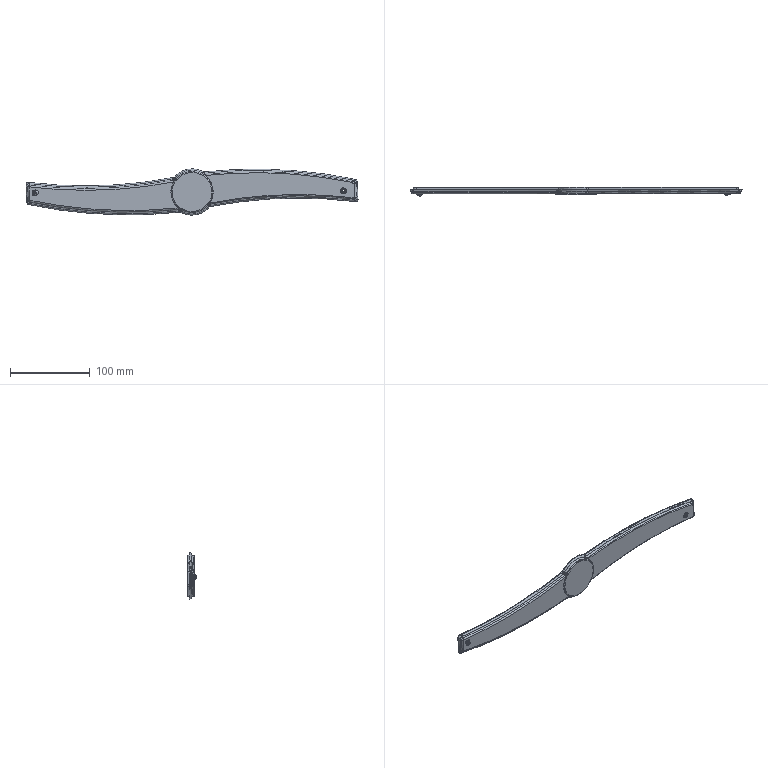Part | STEP file | MSBR-29 | 1 solid | 234 faces | box 415.551 x 11.251 x 58 mm | volume 35121 mm3 | cylinder 77 | spline 76 | torus 48 | plane 19 | other 8 | sphere 6 | commonest cylinder face diameters 4 x11 2 x8 6 x8 1 x6 9 x4 10 x4